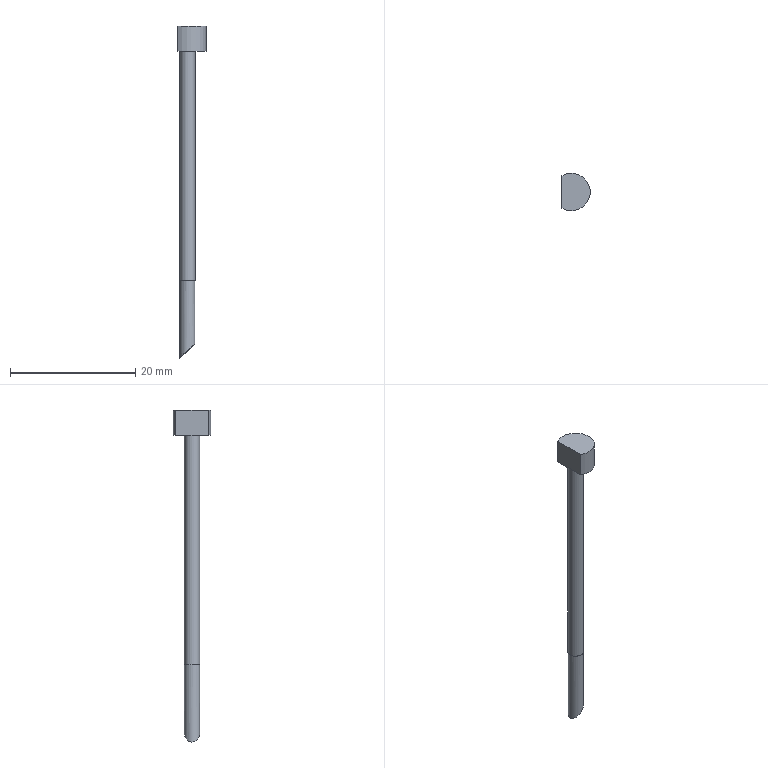Part | NX | features solid 2 | 1 solid | 8 faces | box 4.5 x 6 x 53.083 mm | volume 322.196 mm3 | cylinder 4 | plane 4 | commonest cylinder face diameters 2.412 x1 2.5 x1 6 x1 26.633 x1
STEP:
#1=CARTESIAN_POINT('',(-10.383,23.872,66.5));
#2=VERTEX_POINT('',#1);
#3=CARTESIAN_POINT('',(-10.383,23.872,70.5));
#4=VERTEX_POINT('',#3);
#5=CARTESIAN_POINT('',(-10.383,23.872,66.5));
#6=DIRECTION('',(0.,0.,1.));
#7=VECTOR('',#6,1000.);
#8=LINE('',#5,#7);
#9=EDGE_CURVE('',#2,#4,#8,.T.);
#10=ORIENTED_EDGE('',*,*,#9,.F.);
#11=CARTESIAN_POINT('',(-10.383,29.069,66.5));
#12=VERTEX_POINT('',#11);
#13=CARTESIAN_POINT('',(-8.883,26.471,66.5));
#14=DIRECTION('',(0.,0.,-1.));
#15=DIRECTION('',(-1.,0.,0.));
#16=AXIS2_PLACEMENT_3D('',#13,#14,#15);
#17=CIRCLE('',#16,3.);
#18=EDGE_CURVE('',#12,#2,#17,.T.);
#19=ORIENTED_EDGE('',*,*,#18,.F.);
#20=CARTESIAN_POINT('',(-10.383,29.069,70.5));
#21=VERTEX_POINT('',#20);
#22=CARTESIAN_POINT('',(-10.383,29.069,66.5));
#23=DIRECTION('',(0.,0.,1.));
#24=VECTOR('',#23,1000.);
#25=LINE('',#22,#24);
#26=EDGE_CURVE('',#21,#12,#25,.F.);
#27=ORIENTED_EDGE('',*,*,#26,.F.);
#28=CARTESIAN_POINT('',(-8.883,26.471,70.5));
#29=DIRECTION('',(0.,0.,-1.));
#30=DIRECTION('',(-1.,0.,0.));
#31=AXIS2_PLACEMENT_3D('',#28,#29,#30);
#32=CIRCLE('',#31,3.);
#33=EDGE_CURVE('',#21,#4,#32,.T.);
#34=ORIENTED_EDGE('',*,*,#33,.T.);
#35=EDGE_LOOP('',(#10,#19,#27,#34));
#36=FACE_BOUND('',#35,.T.);
#37=CARTESIAN_POINT('',(-8.883,26.471,66.5));
#38=DIRECTION('',(0.,0.,1.));
#39=DIRECTION('',(1.,0.,0.));
#40=AXIS2_PLACEMENT_3D('',#37,#38,#39);
#41=CYLINDRICAL_SURFACE('',#40,3.);
#42=ADVANCED_FACE('',(#36),#41,.T.);
#43=CARTESIAN_POINT('',(-10.133,26.471,66.5));
#44=VERTEX_POINT('',#43);
#45=CARTESIAN_POINT('',(-8.883,26.471,66.5));
#46=DIRECTION('',(0.,0.,-1.));
#47=DIRECTION('',(-1.,0.,0.));
#48=AXIS2_PLACEMENT_3D('',#45,#46,#47);
#49=CIRCLE('',#48,1.25);
#50=EDGE_CURVE('',#44,#44,#49,.F.);
#51=ORIENTED_EDGE('',*,*,#50,.T.);
#52=EDGE_LOOP('',(#51));
#53=FACE_BOUND('',#52,.T.);
#54=ORIENTED_EDGE('',*,*,#18,.T.);
#55=CARTESIAN_POINT('',(-10.383,26.471,66.5));
#56=DIRECTION('',(0.,1.,0.));
#57=VECTOR('',#56,1000.);
#58=LINE('',#55,#57);
#59=EDGE_CURVE('',#2,#12,#58,.T.);
#60=ORIENTED_EDGE('',*,*,#59,.T.);
#61=EDGE_LOOP('',(#54,#60));
#62=FACE_BOUND('',#61,.T.);
#63=CARTESIAN_POINT('',(-8.883,26.471,66.5));
#64=DIRECTION('',(0.,0.,-1.));
#65=DIRECTION('',(-1.,0.,0.));
#66=AXIS2_PLACEMENT_3D('',#63,#64,#65);
#67=PLANE('',#66);
#68=ADVANCED_FACE('',(#53,#62),#67,.T.);
#69=ORIENTED_EDGE('',*,*,#33,.F.);
#70=CARTESIAN_POINT('',(-10.383,0.,70.5));
#71=DIRECTION('',(0.,-1.,0.));
#72=VECTOR('',#71,1000.);
#73=LINE('',#70,#72);
#74=EDGE_CURVE('',#21,#4,#73,.T.);
#75=ORIENTED_EDGE('',*,*,#74,.T.);
#76=EDGE_LOOP('',(#69,#75));
#77=FACE_BOUND('',#76,.T.);
#78=CARTESIAN_POINT('',(0.,0.,70.5));
#79=DIRECTION('',(0.,0.,1.));
#80=DIRECTION('',(1.,0.,0.));
#81=AXIS2_PLACEMENT_3D('',#78,#79,#80);
#82=PLANE('',#81);
#83=ADVANCED_FACE('',(#77),#82,.T.);
#84=CARTESIAN_POINT('',(-8.883,25.265,18.646));
#85=VERTEX_POINT('',#84);
#86=CARTESIAN_POINT('',(-9.561,25.403,18.004));
#87=CARTESIAN_POINT('',(-8.899,25.175,18.656));
#88=CARTESIAN_POINT('',(-8.01,25.438,19.377));
#89=CARTESIAN_POINT('',(-7.487,26.548,19.738));
#90=CARTESIAN_POINT('',(-8.116,27.575,19.299));
#91=CARTESIAN_POINT('',(-9.,27.757,18.563));
#92=CARTESIAN_POINT('',(-9.646,27.484,17.915));
#93=CARTESIAN_POINT('',(-10.024,26.968,17.493));
#94=CARTESIAN_POINT('',(-10.133,26.399,17.364));
#95=CARTESIAN_POINT('',(-9.966,25.865,17.56));
#96=CARTESIAN_POINT('',(-9.561,25.403,18.004));
#97=CARTESIAN_POINT('',(-8.899,25.175,18.656));
#98=CARTESIAN_POINT('',(-8.01,25.438,19.377));
#99=B_SPLINE_CURVE_WITH_KNOTS('',3,(#86,#87,#88,#89,#90,#91,#92,#93,#94,#95,#96,#97,#98),.UNSPECIFIED.,.T.,.F.,(1,1,1,1,1,1,1,1,1,1,1,1,1,1,1,1,1),(-0.002226,-0.00167,-0.001113,0.,0.001113,0.002226,0.003339,0.004452,0.005565,0.006122,0.006678,0.007235,0.007791,0.008905,0.01002,0.01113,0.01224),.UNSPECIFIED.);
#100=EDGE_CURVE('',#85,#85,#99,.F.);
#101=ORIENTED_EDGE('',*,*,#100,.T.);
#102=EDGE_LOOP('',(#101));
#103=FACE_BOUND('',#102,.T.);
#104=CARTESIAN_POINT('',(0.,0.,8.725));
#105=DIRECTION('',(0.,-1.,0.));
#106=DIRECTION('',(1.,0.,0.));
#107=AXIS2_PLACEMENT_3D('',#104,#105,#106);
#108=CYLINDRICAL_SURFACE('',#107,13.316);
#109=ADVANCED_FACE('',(#103),#108,.F.);
#110=CARTESIAN_POINT('',(-7.841,27.078,29.83));
#111=VERTEX_POINT('',#110);
#112=CARTESIAN_POINT('',(-8.883,26.471,29.83));
#113=DIRECTION('',(0.,0.,1.));
#114=DIRECTION('',(0.8637,0.5041,0.));
#115=AXIS2_PLACEMENT_3D('',#112,#113,#114);
#116=CIRCLE('',#115,1.206);
#117=EDGE_CURVE('',#111,#111,#116,.F.);
#118=ORIENTED_EDGE('',*,*,#117,.T.);
#119=EDGE_LOOP('',(#118));
#120=FACE_BOUND('',#119,.T.);
#121=ORIENTED_EDGE('',*,*,#100,.F.);
#122=EDGE_LOOP('',(#121));
#123=FACE_BOUND('',#122,.T.);
#124=CARTESIAN_POINT('',(-8.883,26.471,31.84));
#125=DIRECTION('',(0.,0.,1.));
#126=DIRECTION('',(0.,-1.,0.));
#127=AXIS2_PLACEMENT_3D('',#124,#125,#126);
#128=CYLINDRICAL_SURFACE('',#127,1.206);
#129=ADVANCED_FACE('',(#120,#123),#128,.T.);
#130=CARTESIAN_POINT('',(-7.633,26.471,29.83));
#131=VERTEX_POINT('',#130);
#132=CARTESIAN_POINT('',(-8.883,26.471,29.83));
#133=DIRECTION('',(0.,0.,1.));
#134=DIRECTION('',(1.,0.,0.));
#135=AXIS2_PLACEMENT_3D('',#132,#133,#134);
#136=CIRCLE('',#135,1.25);
#137=EDGE_CURVE('',#131,#131,#136,.F.);
#138=ORIENTED_EDGE('',*,*,#137,.T.);
#139=EDGE_LOOP('',(#138));
#140=FACE_BOUND('',#139,.T.);
#141=ORIENTED_EDGE('',*,*,#117,.F.);
#142=EDGE_LOOP('',(#141));
#143=FACE_BOUND('',#142,.T.);
#144=CARTESIAN_POINT('',(0.,0.,29.83));
#145=DIRECTION('',(0.,0.,1.));
#146=DIRECTION('',(0.,-1.,0.));
#147=AXIS2_PLACEMENT_3D('',#144,#145,#146);
#148=PLANE('',#147);
#149=ADVANCED_FACE('',(#140,#143),#148,.F.);
#150=ORIENTED_EDGE('',*,*,#50,.F.);
#151=EDGE_LOOP('',(#150));
#152=FACE_BOUND('',#151,.T.);
#153=ORIENTED_EDGE('',*,*,#137,.F.);
#154=EDGE_LOOP('',(#153));
#155=FACE_BOUND('',#154,.T.);
#156=CARTESIAN_POINT('',(-8.883,26.471,108.83));
#157=DIRECTION('',(0.,0.,-1.));
#158=DIRECTION('',(-1.,0.,0.));
#159=AXIS2_PLACEMENT_3D('',#156,#157,#158);
#160=CYLINDRICAL_SURFACE('',#159,1.25);
#161=ADVANCED_FACE('',(#152,#155),#160,.T.);
#162=ORIENTED_EDGE('',*,*,#59,.F.);
#163=ORIENTED_EDGE('',*,*,#9,.T.);
#164=ORIENTED_EDGE('',*,*,#74,.F.);
#165=ORIENTED_EDGE('',*,*,#26,.T.);
#166=EDGE_LOOP('',(#162,#163,#164,#165));
#167=FACE_BOUND('',#166,.T.);
#168=CARTESIAN_POINT('',(-10.383,17.587,43.14));
#169=DIRECTION('',(-1.,0.,0.));
#170=DIRECTION('',(0.,0.,1.));
#171=AXIS2_PLACEMENT_3D('',#168,#169,#170);
#172=PLANE('',#171);
#173=ADVANCED_FACE('',(#167),#172,.T.);
#174=CLOSED_SHELL('',(#42,#68,#83,#109,#129,#149,#161,#173));
#175=MANIFOLD_SOLID_BREP('',#174);
#176=(LENGTH_UNIT()NAMED_UNIT(*)SI_UNIT(.MILLI.,.METRE.));
#177=UNCERTAINTY_MEASURE_WITH_UNIT(LENGTH_MEASURE(0.0508),#176,'','');
#178=(NAMED_UNIT(*)PLANE_ANGLE_UNIT()SI_UNIT($,.RADIAN.));
#179=(NAMED_UNIT(*)SI_UNIT($,.STERADIAN.)SOLID_ANGLE_UNIT());
#180=(GEOMETRIC_REPRESENTATION_CONTEXT(3)GLOBAL_UNCERTAINTY_ASSIGNED_CONTEXT((#177))GLOBAL_UNIT_ASSIGNED_CONTEXT((#176,#178,#179))REPRESENTATION_CONTEXT('',''));
#181=ADVANCED_BREP_SHAPE_REPRESENTATION('',(#175),#180);